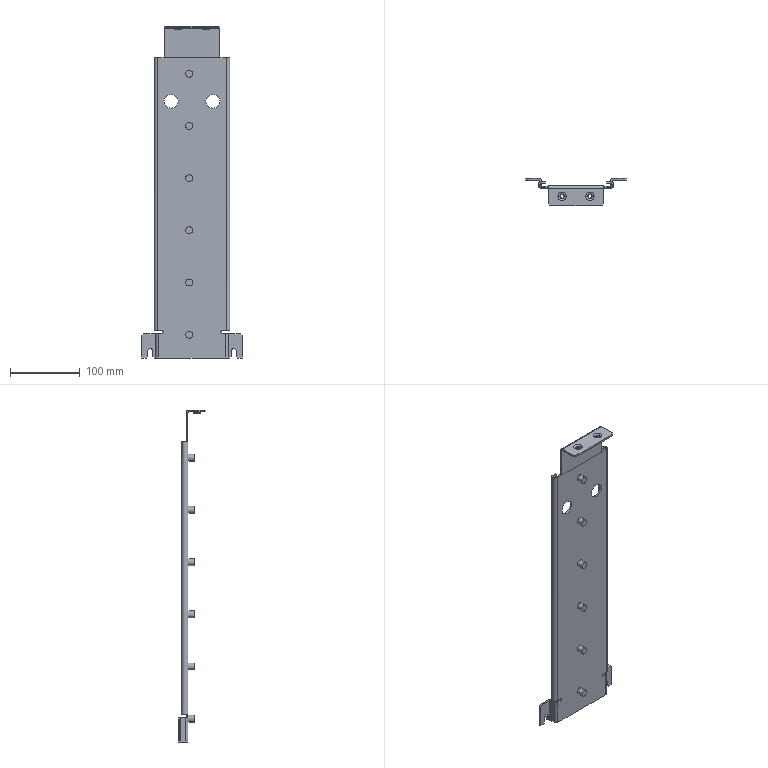Part | STEP file | 64728377 | 1 solid | 147 faces | box 144 x 40.05 x 477.1 mm | volume 161672 mm3 | plane 89 | cylinder 42 | torus 16 | commonest cylinder face diameters 10 x16 1.6 x4 4 x4 5 x4 6.6 x4 20 x4